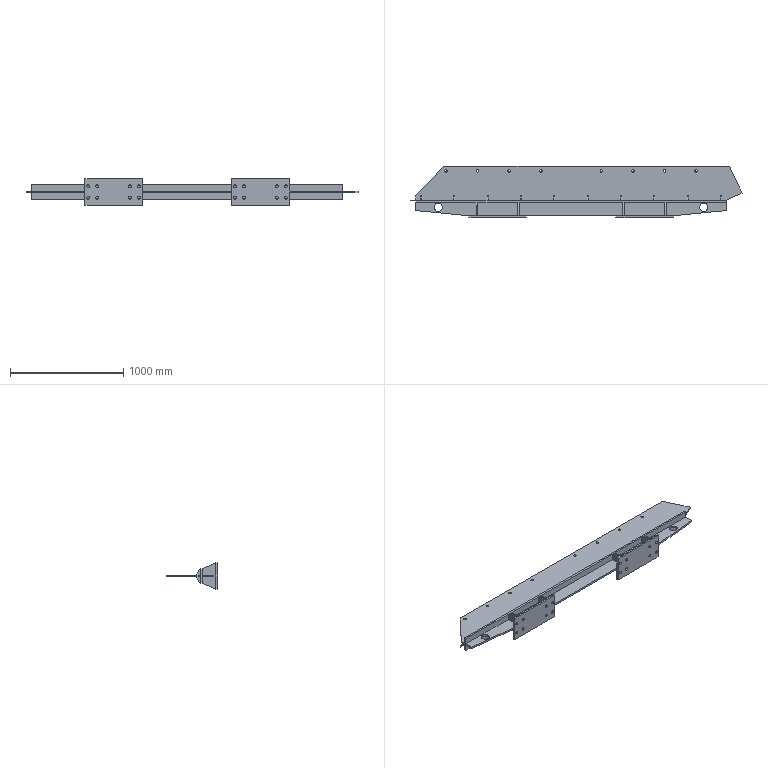Part | STEP file | Screen plate bracket (middle 2)_Default<As machined> | 32 solids | 235 faces | box 2936 x 451.736 x 230 mm | volume 28253471 mm3 | plane 183 | cylinder 52 | commonest cylinder face diameters 25 x32 21.987 x16 71.958 x4